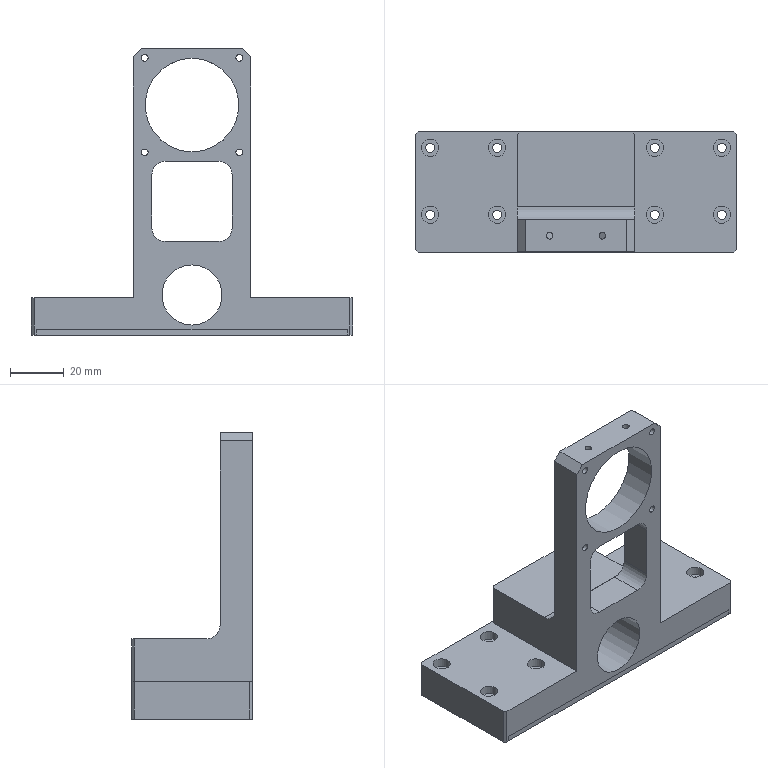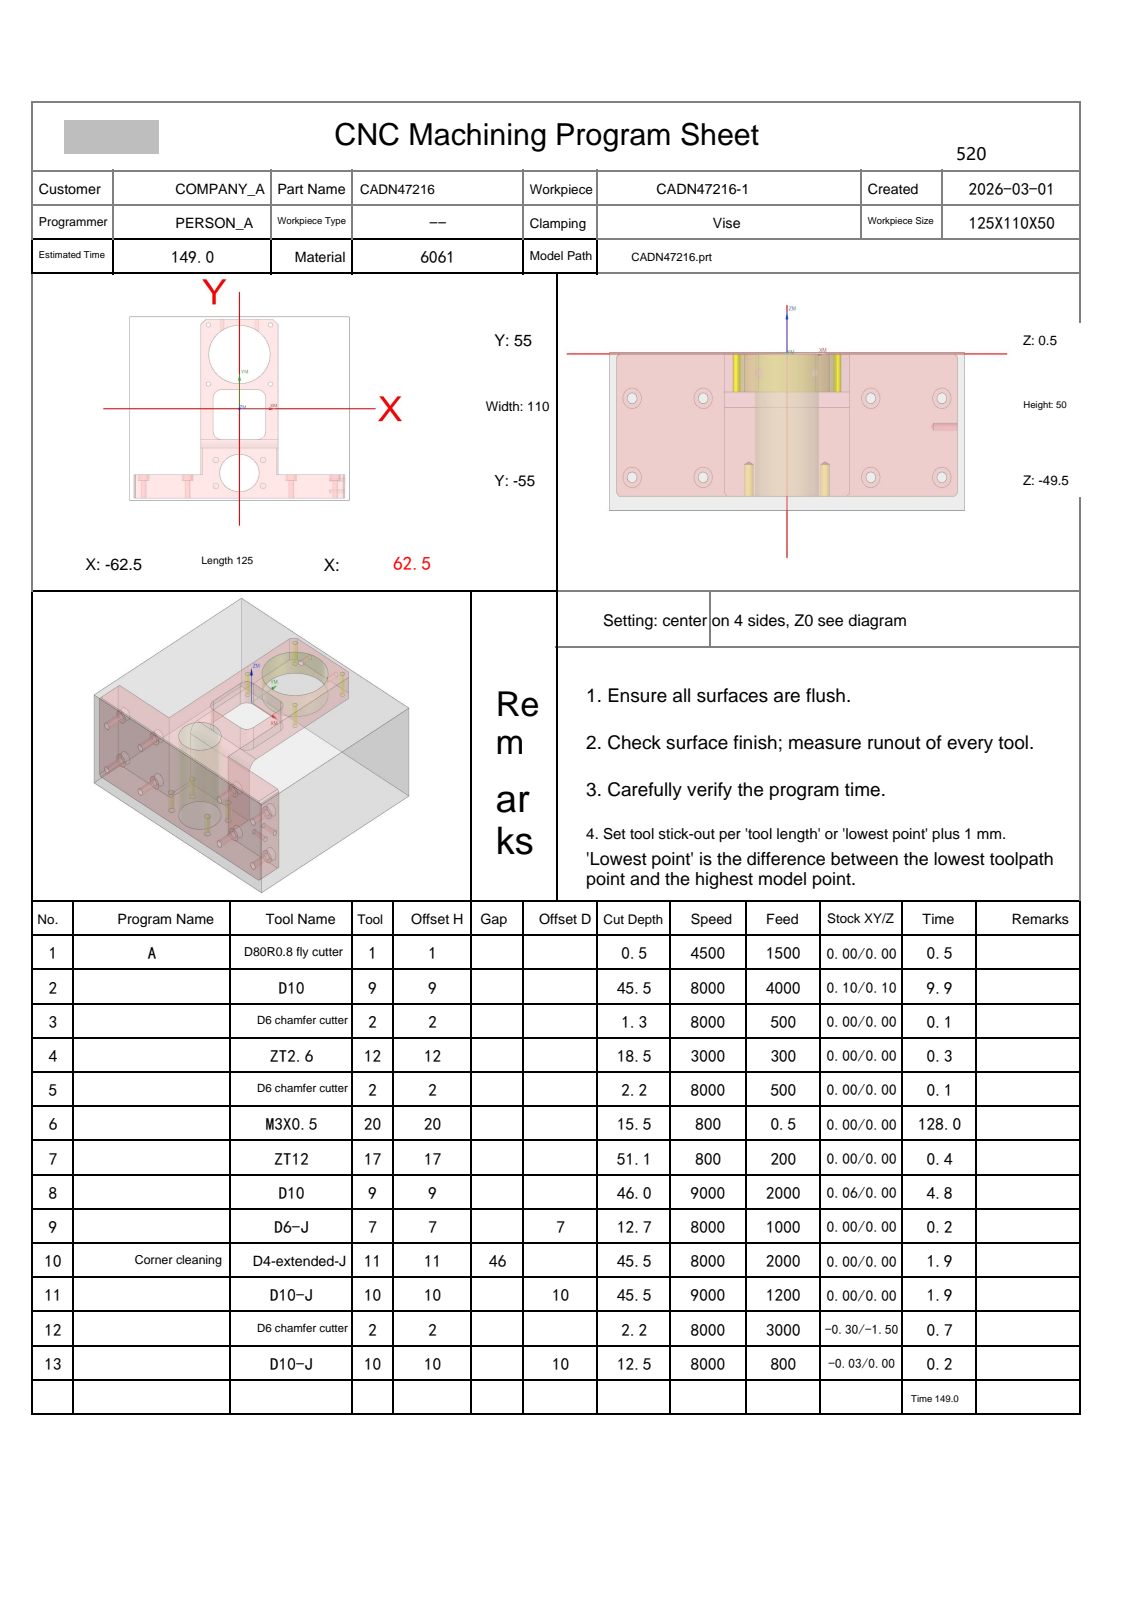NC program | NX | posted by the shop | part box 120 x 45 x 107 mm
Lines 1 to 39 of 16292:
%
O0001
(Machine time: 271.47 MIN)
(===Total Tool:9===)
(T1=D80R0.8 fly cutter D=80.  R=0.8  D-  H01 Z=0.    )
(T9=D10     D=10.  R=0.   D-  H09 Z=-45.5 )
(T2=D6 chamfer cutter   D=6.   R=0.   D-  H02 Z=-1.75 )
(T12=ZT2.6  D=2.6  DR_a=118 D-  H12 Z=-18.  )
(T20=M3X0.5 D=2.5  DR_a=180 D-  H20 Z=-15.  )
(T17=ZT12   D=12.  DR_a=118 D-  H17 Z=-50.61)
(T7=D6-J    D=6.   R=0.   D7  H07 Z=-12.2 )
(T11=D4-extended-J D=4.   R=0.   D-  H11 Z=-45.  )
(T10=D10-J  D=10.  R=0.   D10 H10 Z=-45.  )
G80 G90 G17 G49 G40
G91 G28 Z0
M01
N1 T01 M06
(D80R0.8 fly cutter  D=80. R=0.8 H=01 ce=0.00 di=0.00)
G00 G90 G54 X105. Y-46.75 M03 S4500
G43 H01 Z50.
M08
Z2.
G01 Z0.0 F1500.
X100.
X-100.
Y0.0
X100.
Y46.75
X-100.
X-105.
Z2.
G00 Z50.
G91 G28 Z0.0
M05
M09
G91 G28 Z0.0
M01